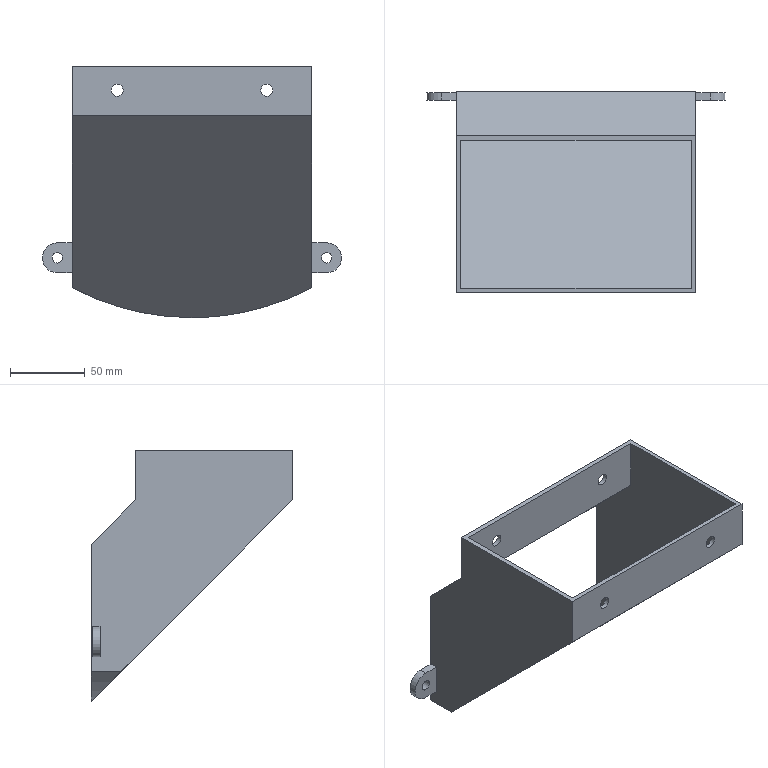Part | NX | features DATUM_CSYS 6, SKETCH 5, EXTRUDE 4, HOLE PACKAGE 4, SIMPLE HOLE 4, BLEND 2, EXTRACT_FACE 2, EXTRACT_STRING 2, DATUM_PLANE 1, Instance Feature 1, Mirror Feature 1, SHELL 1 | 1 solid | 34 faces | box 200 x 135 x 168 mm | volume 211668 mm3 | plane 22 | cylinder 12 | commonest cylinder face diameters 8 x4 7 x2 20 x2 334 x2 340 x2
STEP:
#1=CARTESIAN_POINT('',(160.,135.,-115.));
#2=VERTEX_POINT('',#1);
#3=CARTESIAN_POINT('',(80.,135.,-135.));
#4=VERTEX_POINT('',#3);
#5=CARTESIAN_POINT('',(80.,135.,35.));
#6=DIRECTION('',(0.,-1.,0.));
#7=DIRECTION('',(0.,0.,-1.));
#8=AXIS2_PLACEMENT_3D('',#5,#6,#7);
#9=CIRCLE('',#8,170.);
#10=EDGE_CURVE('',#2,#4,#9,.F.);
#11=ORIENTED_EDGE('',*,*,#10,.T.);
#12=CARTESIAN_POINT('',(0.,135.,-115.));
#13=VERTEX_POINT('',#12);
#14=CARTESIAN_POINT('',(80.,135.,35.));
#15=DIRECTION('',(0.,-1.,0.));
#16=DIRECTION('',(0.,0.,-1.));
#17=AXIS2_PLACEMENT_3D('',#14,#15,#16);
#18=CIRCLE('',#17,170.);
#19=EDGE_CURVE('',#4,#13,#18,.F.);
#20=ORIENTED_EDGE('',*,*,#19,.T.);
#21=CARTESIAN_POINT('',(0.,135.,-30.));
#22=VERTEX_POINT('',#21);
#23=CARTESIAN_POINT('',(0.,135.,-135.));
#24=DIRECTION('',(0.,0.,1.));
#25=VECTOR('',#24,1000.);
#26=LINE('',#23,#25);
#27=EDGE_CURVE('',#13,#22,#26,.T.);
#28=ORIENTED_EDGE('',*,*,#27,.T.);
#29=CARTESIAN_POINT('',(160.,135.,-30.));
#30=VERTEX_POINT('',#29);
#31=CARTESIAN_POINT('',(160.,135.,-30.));
#32=DIRECTION('',(-1.,0.,0.));
#33=VECTOR('',#32,1000.);
#34=LINE('',#31,#33);
#35=EDGE_CURVE('',#30,#22,#34,.T.);
#36=ORIENTED_EDGE('',*,*,#35,.F.);
#37=CARTESIAN_POINT('',(160.,135.,-135.));
#38=DIRECTION('',(0.,0.,1.));
#39=VECTOR('',#38,1000.);
#40=LINE('',#37,#39);
#41=EDGE_CURVE('',#2,#30,#40,.T.);
#42=ORIENTED_EDGE('',*,*,#41,.F.);
#43=EDGE_LOOP('',(#11,#20,#28,#36,#42));
#44=FACE_BOUND('',#43,.T.);
#45=CARTESIAN_POINT('',(157.,135.,-113.189));
#46=VERTEX_POINT('',#45);
#47=CARTESIAN_POINT('',(100.335,135.,-130.757));
#48=VERTEX_POINT('',#47);
#49=CARTESIAN_POINT('',(80.,135.,35.));
#50=DIRECTION('',(0.,-1.,0.));
#51=DIRECTION('',(0.,0.,-1.));
#52=AXIS2_PLACEMENT_3D('',#49,#50,#51);
#53=CIRCLE('',#52,167.);
#54=EDGE_CURVE('',#46,#48,#53,.F.);
#55=ORIENTED_EDGE('',*,*,#54,.F.);
#56=CARTESIAN_POINT('',(157.,135.,-34.243));
#57=VERTEX_POINT('',#56);
#58=CARTESIAN_POINT('',(157.,135.,-135.));
#59=DIRECTION('',(0.,0.,1.));
#60=VECTOR('',#59,1000.);
#61=LINE('',#58,#60);
#62=EDGE_CURVE('',#46,#57,#61,.T.);
#63=ORIENTED_EDGE('',*,*,#62,.T.);
#64=CARTESIAN_POINT('',(3.,135.,-34.243));
#65=VERTEX_POINT('',#64);
#66=CARTESIAN_POINT('',(160.,135.,-34.243));
#67=DIRECTION('',(-1.,0.,0.));
#68=VECTOR('',#67,1000.);
#69=LINE('',#66,#68);
#70=EDGE_CURVE('',#57,#65,#69,.T.);
#71=ORIENTED_EDGE('',*,*,#70,.T.);
#72=CARTESIAN_POINT('',(3.,135.,-113.189));
#73=VERTEX_POINT('',#72);
#74=CARTESIAN_POINT('',(3.,135.,-135.));
#75=DIRECTION('',(0.,0.,1.));
#76=VECTOR('',#75,1000.);
#77=LINE('',#74,#76);
#78=EDGE_CURVE('',#73,#65,#77,.T.);
#79=ORIENTED_EDGE('',*,*,#78,.F.);
#80=CARTESIAN_POINT('',(59.665,135.,-130.757));
#81=VERTEX_POINT('',#80);
#82=CARTESIAN_POINT('',(80.,135.,35.));
#83=DIRECTION('',(0.,-1.,0.));
#84=DIRECTION('',(0.,0.,-1.));
#85=AXIS2_PLACEMENT_3D('',#82,#83,#84);
#86=CIRCLE('',#85,167.);
#87=EDGE_CURVE('',#81,#73,#86,.F.);
#88=ORIENTED_EDGE('',*,*,#87,.F.);
#89=CARTESIAN_POINT('',(160.,135.,-130.757));
#90=DIRECTION('',(-1.,0.,0.));
#91=VECTOR('',#90,1000.);
#92=LINE('',#89,#91);
#93=EDGE_CURVE('',#48,#81,#92,.T.);
#94=ORIENTED_EDGE('',*,*,#93,.F.);
#95=EDGE_LOOP('',(#55,#63,#71,#79,#88,#94));
#96=FACE_BOUND('',#95,.T.);
#97=CARTESIAN_POINT('',(160.,135.,-135.));
#98=DIRECTION('',(0.,-1.,0.));
#99=DIRECTION('',(0.,0.,-1.));
#100=AXIS2_PLACEMENT_3D('',#97,#98,#99);
#101=PLANE('',#100);
#102=ADVANCED_FACE('',(#44,#96),#101,.F.);
#103=CARTESIAN_POINT('',(0.,105.,33.));
#104=VERTEX_POINT('',#103);
#105=CARTESIAN_POINT('',(0.,0.,33.));
#106=VERTEX_POINT('',#105);
#107=CARTESIAN_POINT('',(0.,105.,33.));
#108=DIRECTION('',(0.,-1.,0.));
#109=VECTOR('',#108,1000.);
#110=LINE('',#107,#109);
#111=EDGE_CURVE('',#104,#106,#110,.T.);
#112=ORIENTED_EDGE('',*,*,#111,.T.);
#113=CARTESIAN_POINT('',(160.,0.,33.));
#114=VERTEX_POINT('',#113);
#115=CARTESIAN_POINT('',(160.,0.,33.));
#116=DIRECTION('',(-1.,0.,0.));
#117=VECTOR('',#116,1000.);
#118=LINE('',#115,#117);
#119=EDGE_CURVE('',#114,#106,#118,.T.);
#120=ORIENTED_EDGE('',*,*,#119,.F.);
#121=CARTESIAN_POINT('',(160.,105.,33.));
#122=VERTEX_POINT('',#121);
#123=CARTESIAN_POINT('',(160.,105.,33.));
#124=DIRECTION('',(0.,-1.,0.));
#125=VECTOR('',#124,1000.);
#126=LINE('',#123,#125);
#127=EDGE_CURVE('',#122,#114,#126,.T.);
#128=ORIENTED_EDGE('',*,*,#127,.F.);
#129=CARTESIAN_POINT('',(160.,105.,33.));
#130=DIRECTION('',(-1.,0.,0.));
#131=VECTOR('',#130,1000.);
#132=LINE('',#129,#131);
#133=EDGE_CURVE('',#122,#104,#132,.T.);
#134=ORIENTED_EDGE('',*,*,#133,.T.);
#135=EDGE_LOOP('',(#112,#120,#128,#134));
#136=FACE_BOUND('',#135,.T.);
#137=CARTESIAN_POINT('',(3.,102.,33.));
#138=VERTEX_POINT('',#137);
#139=CARTESIAN_POINT('',(3.,3.,33.));
#140=VERTEX_POINT('',#139);
#141=CARTESIAN_POINT('',(3.,105.,33.));
#142=DIRECTION('',(0.,-1.,0.));
#143=VECTOR('',#142,1000.);
#144=LINE('',#141,#143);
#145=EDGE_CURVE('',#138,#140,#144,.T.);
#146=ORIENTED_EDGE('',*,*,#145,.F.);
#147=CARTESIAN_POINT('',(157.,102.,33.));
#148=VERTEX_POINT('',#147);
#149=CARTESIAN_POINT('',(160.,102.,33.));
#150=DIRECTION('',(-1.,0.,0.));
#151=VECTOR('',#150,1000.);
#152=LINE('',#149,#151);
#153=EDGE_CURVE('',#148,#138,#152,.T.);
#154=ORIENTED_EDGE('',*,*,#153,.F.);
#155=CARTESIAN_POINT('',(157.,3.,33.));
#156=VERTEX_POINT('',#155);
#157=CARTESIAN_POINT('',(157.,105.,33.));
#158=DIRECTION('',(0.,-1.,0.));
#159=VECTOR('',#158,1000.);
#160=LINE('',#157,#159);
#161=EDGE_CURVE('',#148,#156,#160,.T.);
#162=ORIENTED_EDGE('',*,*,#161,.T.);
#163=CARTESIAN_POINT('',(160.,3.,33.));
#164=DIRECTION('',(-1.,0.,0.));
#165=VECTOR('',#164,1000.);
#166=LINE('',#163,#165);
#167=EDGE_CURVE('',#156,#140,#166,.T.);
#168=ORIENTED_EDGE('',*,*,#167,.T.);
#169=EDGE_LOOP('',(#146,#154,#162,#168));
#170=FACE_BOUND('',#169,.T.);
#171=CARTESIAN_POINT('',(160.,105.,33.));
#172=DIRECTION('',(0.,0.,-1.));
#173=DIRECTION('',(-1.,0.,0.));
#174=AXIS2_PLACEMENT_3D('',#171,#172,#173);
#175=PLANE('',#174);
#176=ADVANCED_FACE('',(#136,#170),#175,.F.);
#177=CARTESIAN_POINT('',(130.,3.,21.));
#178=VERTEX_POINT('',#177);
#179=CARTESIAN_POINT('',(130.,3.,17.));
#180=DIRECTION('',(0.,1.,0.));
#181=DIRECTION('',(0.,0.,1.));
#182=AXIS2_PLACEMENT_3D('',#179,#180,#181);
#183=CIRCLE('',#182,4.);
#184=EDGE_CURVE('',#178,#178,#183,.T.);
#185=ORIENTED_EDGE('',*,*,#184,.T.);
#186=EDGE_LOOP('',(#185));
#187=FACE_BOUND('',#186,.T.);
#188=CARTESIAN_POINT('',(130.,0.,21.));
#189=VERTEX_POINT('',#188);
#190=CARTESIAN_POINT('',(130.,0.,17.));
#191=DIRECTION('',(0.,1.,0.));
#192=DIRECTION('',(0.,0.,1.));
#193=AXIS2_PLACEMENT_3D('',#190,#191,#192);
#194=CIRCLE('',#193,4.);
#195=EDGE_CURVE('',#189,#189,#194,.T.);
#196=ORIENTED_EDGE('',*,*,#195,.F.);
#197=EDGE_LOOP('',(#196));
#198=FACE_BOUND('',#197,.T.);
#199=CARTESIAN_POINT('',(130.,0.,17.));
#200=DIRECTION('',(0.,1.,0.));
#201=DIRECTION('',(0.,0.,1.));
#202=AXIS2_PLACEMENT_3D('',#199,#200,#201);
#203=CYLINDRICAL_SURFACE('',#202,4.);
#204=ADVANCED_FACE('',(#187,#198),#203,.F.);
#205=CARTESIAN_POINT('',(30.,3.,21.));
#206=VERTEX_POINT('',#205);
#207=CARTESIAN_POINT('',(30.,3.,17.));
#208=DIRECTION('',(0.,1.,0.));
#209=DIRECTION('',(0.,0.,1.));
#210=AXIS2_PLACEMENT_3D('',#207,#208,#209);
#211=CIRCLE('',#210,4.);
#212=EDGE_CURVE('',#206,#206,#211,.T.);
#213=ORIENTED_EDGE('',*,*,#212,.T.);
#214=EDGE_LOOP('',(#213));
#215=FACE_BOUND('',#214,.T.);
#216=CARTESIAN_POINT('',(30.,0.,21.));
#217=VERTEX_POINT('',#216);
#218=CARTESIAN_POINT('',(30.,0.,17.));
#219=DIRECTION('',(0.,1.,0.));
#220=DIRECTION('',(0.,0.,1.));
#221=AXIS2_PLACEMENT_3D('',#218,#219,#220);
#222=CIRCLE('',#221,4.);
#223=EDGE_CURVE('',#217,#217,#222,.T.);
#224=ORIENTED_EDGE('',*,*,#223,.F.);
#225=EDGE_LOOP('',(#224));
#226=FACE_BOUND('',#225,.T.);
#227=CARTESIAN_POINT('',(30.,0.,17.));
#228=DIRECTION('',(0.,1.,0.));
#229=DIRECTION('',(0.,0.,1.));
#230=AXIS2_PLACEMENT_3D('',#227,#228,#229);
#231=CYLINDRICAL_SURFACE('',#230,4.);
#232=ADVANCED_FACE('',(#215,#226),#231,.F.);
#233=CARTESIAN_POINT('',(0.,0.,0.));
#234=VERTEX_POINT('',#233);
#235=CARTESIAN_POINT('',(0.,115.,-115.));
#236=VERTEX_POINT('',#235);
#237=CARTESIAN_POINT('',(0.,0.,0.));
#238=DIRECTION('',(0.,0.7071,-0.7071));
#239=VECTOR('',#238,1000.);
#240=LINE('',#237,#239);
#241=EDGE_CURVE('',#234,#236,#240,.T.);
#242=ORIENTED_EDGE('',*,*,#241,.T.);
#243=CARTESIAN_POINT('',(80.,-35.,35.));
#244=DIRECTION('',(0.,0.7071,0.7071));
#245=DIRECTION('',(0.,-0.7071,0.7071));
#246=AXIS2_PLACEMENT_3D('',#243,#244,#245);
#247=ELLIPSE('',#246,240.416,170.);
#248=EDGE_CURVE('',#236,#4,#247,.F.);
#249=ORIENTED_EDGE('',*,*,#248,.T.);
#250=CARTESIAN_POINT('',(160.,115.,-115.));
#251=VERTEX_POINT('',#250);
#252=CARTESIAN_POINT('',(80.,-35.,35.));
#253=DIRECTION('',(0.,0.7071,0.7071));
#254=DIRECTION('',(0.,-0.7071,0.7071));
#255=AXIS2_PLACEMENT_3D('',#252,#253,#254);
#256=ELLIPSE('',#255,240.416,170.);
#257=EDGE_CURVE('',#4,#251,#256,.F.);
#258=ORIENTED_EDGE('',*,*,#257,.T.);
#259=CARTESIAN_POINT('',(160.,0.,0.));
#260=VERTEX_POINT('',#259);
#261=CARTESIAN_POINT('',(160.,0.,0.));
#262=DIRECTION('',(0.,0.7071,-0.7071));
#263=VECTOR('',#262,1000.);
#264=LINE('',#261,#263);
#265=EDGE_CURVE('',#260,#251,#264,.T.);
#266=ORIENTED_EDGE('',*,*,#265,.F.);
#267=CARTESIAN_POINT('',(160.,0.,0.));
#268=DIRECTION('',(-1.,0.,0.));
#269=VECTOR('',#268,1000.);
#270=LINE('',#267,#269);
#271=EDGE_CURVE('',#260,#234,#270,.T.);
#272=ORIENTED_EDGE('',*,*,#271,.T.);
#273=EDGE_LOOP('',(#242,#249,#258,#266,#272));
#274=FACE_BOUND('',#273,.T.);
#275=CARTESIAN_POINT('',(160.,0.,0.));
#276=DIRECTION('',(0.,0.7071,0.7071));
#277=DIRECTION('',(0.,-0.7071,0.7071));
#278=AXIS2_PLACEMENT_3D('',#275,#276,#277);
#279=PLANE('',#278);
#280=ADVANCED_FACE('',(#274),#279,.F.);
#281=ORIENTED_EDGE('',*,*,#27,.F.);
#282=CARTESIAN_POINT('',(0.,275.,-115.));
#283=DIRECTION('',(0.,-1.,0.));
#284=VECTOR('',#283,1000.);
#285=LINE('',#282,#284);
#286=EDGE_CURVE('',#13,#236,#285,.T.);
#287=ORIENTED_EDGE('',*,*,#286,.T.);
#288=ORIENTED_EDGE('',*,*,#241,.F.);
#289=CARTESIAN_POINT('',(0.,0.,33.));
#290=DIRECTION('',(0.,0.,-1.));
#291=VECTOR('',#290,1000.);
#292=LINE('',#289,#291);
#293=EDGE_CURVE('',#106,#234,#292,.T.);
#294=ORIENTED_EDGE('',*,*,#293,.F.);
#295=ORIENTED_EDGE('',*,*,#111,.F.);
#296=CARTESIAN_POINT('',(0.,105.,0.));
#297=VERTEX_POINT('',#296);
#298=CARTESIAN_POINT('',(0.,105.,0.));
#299=DIRECTION('',(0.,0.,1.));
#300=VECTOR('',#299,1000.);
#301=LINE('',#298,#300);
#302=EDGE_CURVE('',#297,#104,#301,.T.);
#303=ORIENTED_EDGE('',*,*,#302,.F.);
#304=CARTESIAN_POINT('',(0.,135.,-30.));
#305=DIRECTION('',(0.,-0.7071,0.7071));
#306=VECTOR('',#305,1000.);
#307=LINE('',#304,#306);
#308=EDGE_CURVE('',#22,#297,#307,.T.);
#309=ORIENTED_EDGE('',*,*,#308,.F.);
#310=EDGE_LOOP('',(#281,#287,#288,#294,#295,#303,#309));
#311=FACE_BOUND('',#310,.T.);
#312=CARTESIAN_POINT('',(0.,134.,-85.));
#313=VERTEX_POINT('',#312);
#314=CARTESIAN_POINT('',(0.,134.,-105.));
#315=VERTEX_POINT('',#314);
#316=CARTESIAN_POINT('',(0.,134.,-85.));
#317=DIRECTION('',(0.,0.,-1.));
#318=VECTOR('',#317,1000.);
#319=LINE('',#316,#318);
#320=EDGE_CURVE('',#313,#315,#319,.T.);
#321=ORIENTED_EDGE('',*,*,#320,.F.);
#322=CARTESIAN_POINT('',(0.,129.,-85.));
#323=VERTEX_POINT('',#322);
#324=CARTESIAN_POINT('',(0.,129.,-85.));
#325=DIRECTION('',(0.,1.,0.));
#326=VECTOR('',#325,1000.);
#327=LINE('',#324,#326);
#328=EDGE_CURVE('',#323,#313,#327,.T.);
#329=ORIENTED_EDGE('',*,*,#328,.F.);
#330=CARTESIAN_POINT('',(0.,129.,-105.));
#331=VERTEX_POINT('',#330);
#332=CARTESIAN_POINT('',(0.,129.,-85.));
#333=DIRECTION('',(0.,0.,-1.));
#334=VECTOR('',#333,1000.);
#335=LINE('',#332,#334);
#336=EDGE_CURVE('',#323,#331,#335,.T.);
#337=ORIENTED_EDGE('',*,*,#336,.T.);
#338=CARTESIAN_POINT('',(0.,129.,-105.));
#339=DIRECTION('',(0.,1.,0.));
#340=VECTOR('',#339,1000.);
#341=LINE('',#338,#340);
#342=EDGE_CURVE('',#331,#315,#341,.T.);
#343=ORIENTED_EDGE('',*,*,#342,.T.);
#344=EDGE_LOOP('',(#321,#329,#337,#343));
#345=FACE_BOUND('',#344,.T.);
#346=CARTESIAN_POINT('',(0.,0.,0.));
#347=DIRECTION('',(1.,0.,0.));
#348=DIRECTION('',(0.,0.,-1.));
#349=AXIS2_PLACEMENT_3D('',#346,#347,#348);
#350=PLANE('',#349);
#351=ADVANCED_FACE('',(#311,#345),#350,.F.);
#352=CARTESIAN_POINT('',(160.,275.,-115.));
#353=DIRECTION('',(0.,-1.,0.));
#354=VECTOR('',#353,1000.);
#355=LINE('',#352,#354);
#356=EDGE_CURVE('',#2,#251,#355,.T.);
#357=ORIENTED_EDGE('',*,*,#356,.F.);
#358=ORIENTED_EDGE('',*,*,#41,.T.);
#359=CARTESIAN_POINT('',(160.,105.,0.));
#360=VERTEX_POINT('',#359);
#361=CARTESIAN_POINT('',(160.,135.,-30.));
#362=DIRECTION('',(0.,-0.7071,0.7071));
#363=VECTOR('',#362,1000.);
#364=LINE('',#361,#363);
#365=EDGE_CURVE('',#30,#360,#364,.T.);
#366=ORIENTED_EDGE('',*,*,#365,.T.);
#367=CARTESIAN_POINT('',(160.,105.,0.));
#368=DIRECTION('',(0.,0.,1.));
#369=VECTOR('',#368,1000.);
#370=LINE('',#367,#369);
#371=EDGE_CURVE('',#360,#122,#370,.T.);
#372=ORIENTED_EDGE('',*,*,#371,.T.);
#373=ORIENTED_EDGE('',*,*,#127,.T.);
#374=CARTESIAN_POINT('',(160.,0.,33.));
#375=DIRECTION('',(0.,0.,-1.));
#376=VECTOR('',#375,1000.);
#377=LINE('',#374,#376);
#378=EDGE_CURVE('',#114,#260,#377,.T.);
#379=ORIENTED_EDGE('',*,*,#378,.T.);
#380=ORIENTED_EDGE('',*,*,#265,.T.);
#381=EDGE_LOOP('',(#357,#358,#366,#372,#373,#379,#380));
#382=FACE_BOUND('',#381,.T.);
#383=CARTESIAN_POINT('',(160.,129.,-85.));
#384=VERTEX_POINT('',#383);
#385=CARTESIAN_POINT('',(160.,134.,-85.));
#386=VERTEX_POINT('',#385);
#387=CARTESIAN_POINT('',(160.,129.,-85.));
#388=DIRECTION('',(0.,1.,0.));
#389=VECTOR('',#388,1000.);
#390=LINE('',#387,#389);
#391=EDGE_CURVE('',#384,#386,#390,.T.);
#392=ORIENTED_EDGE('',*,*,#391,.T.);
#393=CARTESIAN_POINT('',(160.,134.,-105.));
#394=VERTEX_POINT('',#393);
#395=CARTESIAN_POINT('',(160.,134.,-85.));
#396=DIRECTION('',(0.,0.,-1.));
#397=VECTOR('',#396,1000.);
#398=LINE('',#395,#397);
#399=EDGE_CURVE('',#386,#394,#398,.T.);
#400=ORIENTED_EDGE('',*,*,#399,.T.);
#401=CARTESIAN_POINT('',(160.,129.,-105.));
#402=VERTEX_POINT('',#401);
#403=CARTESIAN_POINT('',(160.,129.,-105.));
#404=DIRECTION('',(0.,1.,0.));
#405=VECTOR('',#404,1000.);
#406=LINE('',#403,#405);
#407=EDGE_CURVE('',#402,#394,#406,.T.);
#408=ORIENTED_EDGE('',*,*,#407,.F.);
#409=CARTESIAN_POINT('',(160.,129.,-85.));
#410=DIRECTION('',(0.,0.,-1.));
#411=VECTOR('',#410,1000.);
#412=LINE('',#409,#411);
#413=EDGE_CURVE('',#384,#402,#412,.T.);
#414=ORIENTED_EDGE('',*,*,#413,.F.);
#415=EDGE_LOOP('',(#392,#400,#408,#414));
#416=FACE_BOUND('',#415,.T.);
#417=CARTESIAN_POINT('',(160.,0.,0.));
#418=DIRECTION('',(1.,0.,0.));
#419=DIRECTION('',(0.,0.,-1.));
#420=AXIS2_PLACEMENT_3D('',#417,#418,#419);
#421=PLANE('',#420);
#422=ADVANCED_FACE('',(#382,#416),#421,.T.);
#423=ORIENTED_EDGE('',*,*,#223,.T.);
#424=EDGE_LOOP('',(#423));
#425=FACE_BOUND('',#424,.T.);
#426=ORIENTED_EDGE('',*,*,#195,.T.);
#427=EDGE_LOOP('',(#426));
#428=FACE_BOUND('',#427,.T.);
#429=ORIENTED_EDGE('',*,*,#293,.T.);
#430=ORIENTED_EDGE('',*,*,#271,.F.);
#431=ORIENTED_EDGE('',*,*,#378,.F.);
#432=ORIENTED_EDGE('',*,*,#119,.T.);
#433=EDGE_LOOP('',(#429,#430,#431,#432));
#434=FACE_BOUND('',#433,.T.);
#435=CARTESIAN_POINT('',(160.,0.,33.));
#436=DIRECTION('',(0.,1.,0.));
#437=DIRECTION('',(0.,0.,1.));
#438=AXIS2_PLACEMENT_3D('',#435,#436,#437);
#439=PLANE('',#438);
#440=ADVANCED_FACE('',(#425,#428,#434),#439,.F.);
#441=ORIENTED_EDGE('',*,*,#308,.T.);
#442=CARTESIAN_POINT('',(160.,105.,0.));
#443=DIRECTION('',(-1.,0.,0.));
#444=VECTOR('',#443,1000.);
#445=LINE('',#442,#444);
#446=EDGE_CURVE('',#360,#297,#445,.T.);
#447=ORIENTED_EDGE('',*,*,#446,.F.);
#448=ORIENTED_EDGE('',*,*,#365,.F.);
#449=ORIENTED_EDGE('',*,*,#35,.T.);
#450=EDGE_LOOP('',(#441,#447,#448,#449));
#451=FACE_BOUND('',#450,.T.);
#452=CARTESIAN_POINT('',(160.,135.,-30.));
#453=DIRECTION('',(0.,-0.7071,-0.7071));
#454=DIRECTION('',(0.,0.7071,-0.7071));
#455=AXIS2_PLACEMENT_3D('',#452,#453,#454);
#456=PLANE('',#455);
#457=ADVANCED_FACE('',(#451),#456,.F.);
#458=CARTESIAN_POINT('',(30.,105.,13.));
#459=VERTEX_POINT('',#458);
#460=CARTESIAN_POINT('',(30.,105.,17.));
#461=DIRECTION('',(0.,-1.,0.));
#462=DIRECTION('',(0.,0.,-1.));
#463=AXIS2_PLACEMENT_3D('',#460,#461,#462);
#464=CIRCLE('',#463,4.);
#465=EDGE_CURVE('',#459,#459,#464,.T.);
#466=ORIENTED_EDGE('',*,*,#465,.T.);
#467=EDGE_LOOP('',(#466));
#468=FACE_BOUND('',#467,.T.);
#469=CARTESIAN_POINT('',(130.,105.,13.));
#470=VERTEX_POINT('',#469);
#471=CARTESIAN_POINT('',(130.,105.,17.));
#472=DIRECTION('',(0.,-1.,0.));
#473=DIRECTION('',(0.,0.,-1.));
#474=AXIS2_PLACEMENT_3D('',#471,#472,#473);
#475=CIRCLE('',#474,4.);
#476=EDGE_CURVE('',#470,#470,#475,.T.);
#477=ORIENTED_EDGE('',*,*,#476,.T.);
#478=EDGE_LOOP('',(#477));
#479=FACE_BOUND('',#478,.T.);
#480=ORIENTED_EDGE('',*,*,#302,.T.);
#481=ORIENTED_EDGE('',*,*,#133,.F.);
#482=ORIENTED_EDGE('',*,*,#371,.F.);
#483=ORIENTED_EDGE('',*,*,#446,.T.);
#484=EDGE_LOOP('',(#480,#481,#482,#483));
#485=FACE_BOUND('',#484,.T.);
#486=CARTESIAN_POINT('',(160.,105.,0.));
#487=DIRECTION('',(0.,-1.,0.));
#488=DIRECTION('',(0.,0.,-1.));
#489=AXIS2_PLACEMENT_3D('',#486,#487,#488);
#490=PLANE('',#489);
#491=ADVANCED_FACE('',(#468,#479,#485),#490,.F.);
#492=CARTESIAN_POINT('',(170.,129.,-85.));
#493=VERTEX_POINT('',#492);
#494=CARTESIAN_POINT('',(180.,129.,-85.));
#495=DIRECTION('',(-1.,0.,0.));
#496=VECTOR('',#495,1000.);
#497=LINE('',#494,#496);
#498=EDGE_CURVE('',#493,#384,#497,.T.);
#499=ORIENTED_EDGE('',*,*,#498,.F.);
#500=CARTESIAN_POINT('',(170.,134.,-85.));
#501=VERTEX_POINT('',#500);
#502=CARTESIAN_POINT('',(170.,129.,-85.));
#503=DIRECTION('',(0.,1.,0.));
#504=VECTOR('',#503,1000.);
#505=LINE('',#502,#504);
#506=EDGE_CURVE('',#493,#501,#505,.T.);
#507=ORIENTED_EDGE('',*,*,#506,.T.);
#508=CARTESIAN_POINT('',(180.,134.,-85.));
#509=DIRECTION('',(-1.,0.,0.));
#510=VECTOR('',#509,1000.);
#511=LINE('',#508,#510);
#512=EDGE_CURVE('',#501,#386,#511,.T.);
#513=ORIENTED_EDGE('',*,*,#512,.T.);
#514=ORIENTED_EDGE('',*,*,#391,.F.);
#515=EDGE_LOOP('',(#499,#507,#513,#514));
#516=FACE_BOUND('',#515,.T.);
#517=CARTESIAN_POINT('',(180.,129.,-85.));
#518=DIRECTION('',(0.,0.,-1.));
#519=DIRECTION('',(-1.,0.,0.));
#520=AXIS2_PLACEMENT_3D('',#517,#518,#519);
#521=PLANE('',#520);
#522=ADVANCED_FACE('',(#516),#521,.F.);
#523=CARTESIAN_POINT('',(170.,134.,-105.));
#524=VERTEX_POINT('',#523);
#525=CARTESIAN_POINT('',(160.,134.,-105.));
#526=DIRECTION('',(1.,0.,0.));
#527=VECTOR('',#526,1000.);
#528=LINE('',#525,#527);
#529=EDGE_CURVE('',#394,#524,#528,.T.);
#530=ORIENTED_EDGE('',*,*,#529,.T.);
#531=CARTESIAN_POINT('',(170.,129.,-105.));
#532=VERTEX_POINT('',#531);
#533=CARTESIAN_POINT('',(170.,129.,-105.));
#534=DIRECTION('',(0.,1.,0.));
#535=VECTOR('',#534,1000.);
#536=LINE('',#533,#535);
#537=EDGE_CURVE('',#524,#532,#536,.F.);
#538=ORIENTED_EDGE('',*,*,#537,.T.);
#539=CARTESIAN_POINT('',(160.,129.,-105.));
#540=DIRECTION('',(1.,0.,0.));
#541=VECTOR('',#540,1000.);
#542=LINE('',#539,#541);
#543=EDGE_CURVE('',#402,#532,#542,.T.);
#544=ORIENTED_EDGE('',*,*,#543,.F.);
#545=ORIENTED_EDGE('',*,*,#407,.T.);
#546=EDGE_LOOP('',(#530,#538,#544,#545));
#547=FACE_BOUND('',#546,.T.);
#548=CARTESIAN_POINT('',(160.,129.,-105.));
#549=DIRECTION('',(0.,0.,1.));
#550=DIRECTION('',(1.,0.,0.));
#551=AXIS2_PLACEMENT_3D('',#548,#549,#550);
#552=PLANE('',#551);
#553=ADVANCED_FACE('',(#547),#552,.F.);
#554=CARTESIAN_POINT('',(170.,129.,-98.5));
#555=VERTEX_POINT('',#554);
#556=CARTESIAN_POINT('',(170.,129.,-95.));
#557=DIRECTION('',(0.,-1.,0.));
#558=DIRECTION('',(0.,0.,-1.));
#559=AXIS2_PLACEMENT_3D('',#556,#557,#558);
#560=CIRCLE('',#559,3.5);
#561=EDGE_CURVE('',#555,#555,#560,.T.);
#562=ORIENTED_EDGE('',*,*,#561,.F.);
#563=EDGE_LOOP('',(#562));
#564=FACE_BOUND('',#563,.T.);
#565=CARTESIAN_POINT('',(170.,129.,-95.));
#566=DIRECTION('',(0.,-1.,0.));
#567=DIRECTION('',(0.,0.,-1.));
#568=AXIS2_PLACEMENT_3D('',#565,#566,#567);
#569=CIRCLE('',#568,10.);
#570=EDGE_CURVE('',#532,#493,#569,.T.);
#571=ORIENTED_EDGE('',*,*,#570,.T.);
#572=ORIENTED_EDGE('',*,*,#498,.T.);
#573=ORIENTED_EDGE('',*,*,#413,.T.);
#574=ORIENTED_EDGE('',*,*,#543,.T.);
#575=EDGE_LOOP('',(#571,#572,#573,#574));
#576=FACE_BOUND('',#575,.T.);
#577=CARTESIAN_POINT('',(0.,129.,0.));
#578=DIRECTION('',(0.,-1.,0.));
#579=DIRECTION('',(0.,0.,-1.));
#580=AXIS2_PLACEMENT_3D('',#577,#578,#579);
#581=PLANE('',#580);
#582=ADVANCED_FACE('',(#564,#576),#581,.T.);
#583=CARTESIAN_POINT('',(170.,134.,-98.5));
#584=VERTEX_POINT('',#583);
#585=CARTESIAN_POINT('',(170.,134.,-95.));
#586=DIRECTION('',(0.,-1.,0.));
#587=DIRECTION('',(0.,0.,-1.));
#588=AXIS2_PLACEMENT_3D('',#585,#586,#587);
#589=CIRCLE('',#588,3.5);
#590=EDGE_CURVE('',#584,#584,#589,.T.);
#591=ORIENTED_EDGE('',*,*,#590,.T.);
#592=EDGE_LOOP('',(#591));
#593=FACE_BOUND('',#592,.T.);
#594=ORIENTED_EDGE('',*,*,#512,.F.);
#595=CARTESIAN_POINT('',(170.,134.,-95.));
#596=DIRECTION('',(0.,-1.,0.));
#597=DIRECTION('',(0.,0.,-1.));
#598=AXIS2_PLACEMENT_3D('',#595,#596,#597);
#599=CIRCLE('',#598,10.);
#600=EDGE_CURVE('',#501,#524,#599,.F.);
#601=ORIENTED_EDGE('',*,*,#600,.T.);
#602=ORIENTED_EDGE('',*,*,#529,.F.);
#603=ORIENTED_EDGE('',*,*,#399,.F.);
#604=EDGE_LOOP('',(#594,#601,#602,#603));
#605=FACE_BOUND('',#604,.T.);
#606=CARTESIAN_POINT('',(0.,134.,0.));
#607=DIRECTION('',(0.,-1.,0.));
#608=DIRECTION('',(0.,0.,-1.));
#609=AXIS2_PLACEMENT_3D('',#606,#607,#608);
#610=PLANE('',#609);
#611=ADVANCED_FACE('',(#593,#605),#610,.F.);
#612=ORIENTED_EDGE('',*,*,#600,.F.);
#613=ORIENTED_EDGE('',*,*,#506,.F.);
#614=ORIENTED_EDGE('',*,*,#570,.F.);
#615=ORIENTED_EDGE('',*,*,#537,.F.);
#616=EDGE_LOOP('',(#612,#613,#614,#615));
#617=FACE_BOUND('',#616,.T.);
#618=CARTESIAN_POINT('',(170.,129.,-95.));
#619=DIRECTION('',(0.,1.,0.));
#620=DIRECTION('',(0.,0.,1.));
#621=AXIS2_PLACEMENT_3D('',#618,#619,#620);
#622=CYLINDRICAL_SURFACE('',#621,10.);
#623=ADVANCED_FACE('',(#617),#622,.T.);
#624=ORIENTED_EDGE('',*,*,#561,.T.);
#625=EDGE_LOOP('',(#624));
#626=FACE_BOUND('',#625,.T.);
#627=ORIENTED_EDGE('',*,*,#590,.F.);
#628=EDGE_LOOP('',(#627));
#629=FACE_BOUND('',#628,.T.);
#630=CARTESIAN_POINT('',(170.,134.,-95.));
#631=DIRECTION('',(0.,-1.,0.));
#632=DIRECTION('',(0.,0.,-1.));
#633=AXIS2_PLACEMENT_3D('',#630,#631,#632);
#634=CYLINDRICAL_SURFACE('',#633,3.5);
#635=ADVANCED_FACE('',(#626,#629),#634,.F.);
#636=CARTESIAN_POINT('',(130.,102.,13.));
#637=VERTEX_POINT('',#636);
#638=CARTESIAN_POINT('',(130.,102.,17.));
#639=DIRECTION('',(0.,-1.,0.));
#640=DIRECTION('',(0.,0.,-1.));
#641=AXIS2_PLACEMENT_3D('',#638,#639,#640);
#642=CIRCLE('',#641,4.);
#643=EDGE_CURVE('',#637,#637,#642,.T.);
#644=ORIENTED_EDGE('',*,*,#643,.T.);
#645=EDGE_LOOP('',(#644));
#646=FACE_BOUND('',#645,.T.);
#647=ORIENTED_EDGE('',*,*,#476,.F.);
#648=EDGE_LOOP('',(#647));
#649=FACE_BOUND('',#648,.T.);
#650=CARTESIAN_POINT('',(130.,0.,17.));
#651=DIRECTION('',(0.,1.,0.));
#652=DIRECTION('',(0.,0.,1.));
#653=AXIS2_PLACEMENT_3D('',#650,#651,#652);
#654=CYLINDRICAL_SURFACE('',#653,4.);
#655=ADVANCED_FACE('',(#646,#649),#654,.F.);
#656=CARTESIAN_POINT('',(-10.,134.,-85.));
#657=VERTEX_POINT('',#656);
#658=CARTESIAN_POINT('',(-20.,134.,-85.));
#659=DIRECTION('',(1.,0.,0.));
#660=VECTOR('',#659,1000.);
#661=LINE('',#658,#660);
#662=EDGE_CURVE('',#657,#313,#661,.T.);
#663=ORIENTED_EDGE('',*,*,#662,.F.);
#664=CARTESIAN_POINT('',(-10.,129.,-85.));
#665=VERTEX_POINT('',#664);
#666=CARTESIAN_POINT('',(-10.,129.,-85.));
#667=DIRECTION('',(0.,1.,0.));
#668=VECTOR('',#667,1000.);
#669=LINE('',#666,#668);
#670=EDGE_CURVE('',#665,#657,#669,.T.);
#671=ORIENTED_EDGE('',*,*,#670,.F.);
#672=CARTESIAN_POINT('',(-20.,129.,-85.));
#673=DIRECTION('',(1.,0.,0.));
#674=VECTOR('',#673,1000.);
#675=LINE('',#672,#674);
#676=EDGE_CURVE('',#665,#323,#675,.T.);
#677=ORIENTED_EDGE('',*,*,#676,.T.);
#678=ORIENTED_EDGE('',*,*,#328,.T.);
#679=EDGE_LOOP('',(#663,#671,#677,#678));
#680=FACE_BOUND('',#679,.T.);
#681=CARTESIAN_POINT('',(-20.,129.,-85.));
#682=DIRECTION('',(0.,0.,1.));
#683=DIRECTION('',(1.,0.,0.));
#684=AXIS2_PLACEMENT_3D('',#681,#682,#683);
#685=PLANE('',#684);
#686=ADVANCED_FACE('',(#680),#685,.T.);
#687=CARTESIAN_POINT('',(-10.,129.,-105.));
#688=VERTEX_POINT('',#687);
#689=CARTESIAN_POINT('',(0.,129.,-105.));
#690=DIRECTION('',(-1.,0.,0.));
#691=VECTOR('',#690,1000.);
#692=LINE('',#689,#691);
#693=EDGE_CURVE('',#331,#688,#692,.T.);
#694=ORIENTED_EDGE('',*,*,#693,.T.);
#695=CARTESIAN_POINT('',(-10.,134.,-105.));
#696=VERTEX_POINT('',#695);
#697=CARTESIAN_POINT('',(-10.,129.,-105.));
#698=DIRECTION('',(0.,1.,0.));
#699=VECTOR('',#698,1000.);
#700=LINE('',#697,#699);
#701=EDGE_CURVE('',#696,#688,#700,.F.);
#702=ORIENTED_EDGE('',*,*,#701,.F.);
#703=CARTESIAN_POINT('',(0.,134.,-105.));
#704=DIRECTION('',(-1.,0.,0.));
#705=VECTOR('',#704,1000.);
#706=LINE('',#703,#705);
#707=EDGE_CURVE('',#315,#696,#706,.T.);
#708=ORIENTED_EDGE('',*,*,#707,.F.);
#709=ORIENTED_EDGE('',*,*,#342,.F.);
#710=EDGE_LOOP('',(#694,#702,#708,#709));
#711=FACE_BOUND('',#710,.T.);
#712=CARTESIAN_POINT('',(0.,129.,-105.));
#713=DIRECTION('',(0.,0.,-1.));
#714=DIRECTION('',(-1.,0.,0.));
#715=AXIS2_PLACEMENT_3D('',#712,#713,#714);
#716=PLANE('',#715);
#717=ADVANCED_FACE('',(#711),#716,.T.);
#718=CARTESIAN_POINT('',(-10.,129.,-91.5));
#719=VERTEX_POINT('',#718);
#720=CARTESIAN_POINT('',(-10.,129.,-95.));
#721=DIRECTION('',(0.,1.,0.));
#722=DIRECTION('',(0.,0.,1.));
#723=AXIS2_PLACEMENT_3D('',#720,#721,#722);
#724=CIRCLE('',#723,3.5);
#725=EDGE_CURVE('',#719,#719,#724,.T.);
#726=ORIENTED_EDGE('',*,*,#725,.T.);
#727=EDGE_LOOP('',(#726));
#728=FACE_BOUND('',#727,.T.);
#729=ORIENTED_EDGE('',*,*,#676,.F.);
#730=CARTESIAN_POINT('',(-10.,129.,-95.));
#731=DIRECTION('',(0.,1.,0.));
#732=DIRECTION('',(0.,0.,1.));
#733=AXIS2_PLACEMENT_3D('',#730,#731,#732);
#734=CIRCLE('',#733,10.);
#735=EDGE_CURVE('',#688,#665,#734,.T.);
#736=ORIENTED_EDGE('',*,*,#735,.F.);
#737=ORIENTED_EDGE('',*,*,#693,.F.);
#738=ORIENTED_EDGE('',*,*,#336,.F.);
#739=EDGE_LOOP('',(#729,#736,#737,#738));
#740=FACE_BOUND('',#739,.T.);
#741=CARTESIAN_POINT('',(0.,129.,0.));
#742=DIRECTION('',(0.,1.,0.));
#743=DIRECTION('',(0.,0.,1.));
#744=AXIS2_PLACEMENT_3D('',#741,#742,#743);
#745=PLANE('',#744);
#746=ADVANCED_FACE('',(#728,#740),#745,.F.);
#747=CARTESIAN_POINT('',(-10.,134.,-98.5));
#748=VERTEX_POINT('',#747);
#749=CARTESIAN_POINT('',(-10.,134.,-95.));
#750=DIRECTION('',(0.,-1.,0.));
#751=DIRECTION('',(0.,0.,-1.));
#752=AXIS2_PLACEMENT_3D('',#749,#750,#751);
#753=CIRCLE('',#752,3.5);
#754=EDGE_CURVE('',#748,#748,#753,.F.);
#755=ORIENTED_EDGE('',*,*,#754,.F.);
#756=EDGE_LOOP('',(#755));
#757=FACE_BOUND('',#756,.T.);
#758=CARTESIAN_POINT('',(-10.,134.,-95.));
#759=DIRECTION('',(0.,1.,0.));
#760=DIRECTION('',(0.,0.,1.));
#761=AXIS2_PLACEMENT_3D('',#758,#759,#760);
#762=CIRCLE('',#761,10.);
#763=EDGE_CURVE('',#657,#696,#762,.F.);
#764=ORIENTED_EDGE('',*,*,#763,.F.);
#765=ORIENTED_EDGE('',*,*,#662,.T.);
#766=ORIENTED_EDGE('',*,*,#320,.T.);
#767=ORIENTED_EDGE('',*,*,#707,.T.);
#768=EDGE_LOOP('',(#764,#765,#766,#767));
#769=FACE_BOUND('',#768,.T.);
#770=CARTESIAN_POINT('',(0.,134.,0.));
#771=DIRECTION('',(0.,1.,0.));
#772=DIRECTION('',(0.,0.,1.));
#773=AXIS2_PLACEMENT_3D('',#770,#771,#772);
#774=PLANE('',#773);
#775=ADVANCED_FACE('',(#757,#769),#774,.T.);
#776=ORIENTED_EDGE('',*,*,#701,.T.);
#777=ORIENTED_EDGE('',*,*,#735,.T.);
#778=ORIENTED_EDGE('',*,*,#670,.T.);
#779=ORIENTED_EDGE('',*,*,#763,.T.);
#780=EDGE_LOOP('',(#776,#777,#778,#779));
#781=FACE_BOUND('',#780,.T.);
#782=CARTESIAN_POINT('',(-10.,129.,-95.));
#783=DIRECTION('',(0.,1.,0.));
#784=DIRECTION('',(0.,0.,1.));
#785=AXIS2_PLACEMENT_3D('',#782,#783,#784);
#786=CYLINDRICAL_SURFACE('',#785,10.);
#787=ADVANCED_FACE('',(#781),#786,.T.);
#788=ORIENTED_EDGE('',*,*,#754,.T.);
#789=EDGE_LOOP('',(#788));
#790=FACE_BOUND('',#789,.T.);
#791=ORIENTED_EDGE('',*,*,#725,.F.);
#792=EDGE_LOOP('',(#791));
#793=FACE_BOUND('',#792,.T.);
#794=CARTESIAN_POINT('',(-10.,134.,-95.));
#795=DIRECTION('',(0.,-1.,0.));
#796=DIRECTION('',(0.,0.,-1.));
#797=AXIS2_PLACEMENT_3D('',#794,#795,#796);
#798=CYLINDRICAL_SURFACE('',#797,3.5);
#799=ADVANCED_FACE('',(#790,#793),#798,.F.);
#800=CARTESIAN_POINT('',(30.,102.,13.));
#801=VERTEX_POINT('',#800);
#802=CARTESIAN_POINT('',(30.,102.,17.));
#803=DIRECTION('',(0.,-1.,0.));
#804=DIRECTION('',(0.,0.,-1.));
#805=AXIS2_PLACEMENT_3D('',#802,#803,#804);
#806=CIRCLE('',#805,4.);
#807=EDGE_CURVE('',#801,#801,#806,.T.);
#808=ORIENTED_EDGE('',*,*,#807,.T.);
#809=EDGE_LOOP('',(#808));
#810=FACE_BOUND('',#809,.T.);
#811=ORIENTED_EDGE('',*,*,#465,.F.);
#812=EDGE_LOOP('',(#811));
#813=FACE_BOUND('',#812,.T.);
#814=CARTESIAN_POINT('',(30.,0.,17.));
#815=DIRECTION('',(0.,1.,0.));
#816=DIRECTION('',(0.,0.,1.));
#817=AXIS2_PLACEMENT_3D('',#814,#815,#816);
#818=CYLINDRICAL_SURFACE('',#817,4.);
#819=ADVANCED_FACE('',(#810,#813),#818,.F.);
#820=ORIENTED_EDGE('',*,*,#10,.F.);
#821=ORIENTED_EDGE('',*,*,#356,.T.);
#822=ORIENTED_EDGE('',*,*,#257,.F.);
#823=EDGE_LOOP('',(#820,#821,#822));
#824=FACE_BOUND('',#823,.T.);
#825=CARTESIAN_POINT('',(80.,275.,35.));
#826=DIRECTION('',(0.,-1.,0.));
#827=DIRECTION('',(0.,0.,-1.));
#828=AXIS2_PLACEMENT_3D('',#825,#826,#827);
#829=CYLINDRICAL_SURFACE('',#828,170.);
#830=ADVANCED_FACE('',(#824),#829,.T.);
#831=ORIENTED_EDGE('',*,*,#286,.F.);
#832=ORIENTED_EDGE('',*,*,#19,.F.);
#833=ORIENTED_EDGE('',*,*,#248,.F.);
#834=EDGE_LOOP('',(#831,#832,#833));
#835=FACE_BOUND('',#834,.T.);
#836=CARTESIAN_POINT('',(80.,275.,35.));
#837=DIRECTION('',(0.,-1.,0.));
#838=DIRECTION('',(0.,0.,-1.));
#839=AXIS2_PLACEMENT_3D('',#836,#837,#838);
#840=CYLINDRICAL_SURFACE('',#839,170.);
#841=ADVANCED_FACE('',(#835),#840,.T.);
#842=CARTESIAN_POINT('',(3.,3.,1.243));
#843=VERTEX_POINT('',#842);
#844=CARTESIAN_POINT('',(3.,117.432,-113.189));
#845=VERTEX_POINT('',#844);
#846=CARTESIAN_POINT('',(3.,2.121,2.121));
#847=DIRECTION('',(0.,0.7071,-0.7071));
#848=VECTOR('',#847,1000.);
#849=LINE('',#846,#848);
#850=EDGE_CURVE('',#843,#845,#849,.T.);
#851=ORIENTED_EDGE('',*,*,#850,.F.);
#852=CARTESIAN_POINT('',(157.,3.,1.243));
#853=VERTEX_POINT('',#852);
#854=CARTESIAN_POINT('',(160.,3.,1.243));
#855=DIRECTION('',(-1.,0.,0.));
#856=VECTOR('',#855,1000.);
#857=LINE('',#854,#856);
#858=EDGE_CURVE('',#853,#843,#857,.T.);
#859=ORIENTED_EDGE('',*,*,#858,.F.);
#860=CARTESIAN_POINT('',(157.,117.432,-113.189));
#861=VERTEX_POINT('',#860);
#862=CARTESIAN_POINT('',(157.,2.121,2.121));
#863=DIRECTION('',(0.,0.7071,-0.7071));
#864=VECTOR('',#863,1000.);
#865=LINE('',#862,#864);
#866=EDGE_CURVE('',#853,#861,#865,.T.);
#867=ORIENTED_EDGE('',*,*,#866,.T.);
#868=CARTESIAN_POINT('',(80.,-30.757,35.));
#869=DIRECTION('',(0.,0.7071,0.7071));
#870=DIRECTION('',(0.,-0.7071,0.7071));
#871=AXIS2_PLACEMENT_3D('',#868,#869,#870);
#872=ELLIPSE('',#871,236.174,167.);
#873=EDGE_CURVE('',#48,#861,#872,.F.);
#874=ORIENTED_EDGE('',*,*,#873,.F.);
#875=ORIENTED_EDGE('',*,*,#93,.T.);
#876=CARTESIAN_POINT('',(80.,-30.757,35.));
#877=DIRECTION('',(0.,0.7071,0.7071));
#878=DIRECTION('',(0.,-0.7071,0.7071));
#879=AXIS2_PLACEMENT_3D('',#876,#877,#878);
#880=ELLIPSE('',#879,236.174,167.);
#881=EDGE_CURVE('',#845,#81,#880,.F.);
#882=ORIENTED_EDGE('',*,*,#881,.F.);
#883=EDGE_LOOP('',(#851,#859,#867,#874,#875,#882));
#884=FACE_BOUND('',#883,.T.);
#885=CARTESIAN_POINT('',(160.,2.121,2.121));
#886=DIRECTION('',(0.,0.7071,0.7071));
#887=DIRECTION('',(0.,-0.7071,0.7071));
#888=AXIS2_PLACEMENT_3D('',#885,#886,#887);
#889=PLANE('',#888);
#890=ADVANCED_FACE('',(#884),#889,.T.);
#891=ORIENTED_EDGE('',*,*,#78,.T.);
#892=CARTESIAN_POINT('',(3.,102.,-1.243));
#893=VERTEX_POINT('',#892);
#894=CARTESIAN_POINT('',(3.,132.879,-32.121));
#895=DIRECTION('',(0.,-0.7071,0.7071));
#896=VECTOR('',#895,1000.);
#897=LINE('',#894,#896);
#898=EDGE_CURVE('',#65,#893,#897,.T.);
#899=ORIENTED_EDGE('',*,*,#898,.T.);
#900=CARTESIAN_POINT('',(3.,102.,0.));
#901=DIRECTION('',(0.,0.,1.));
#902=VECTOR('',#901,1000.);
#903=LINE('',#900,#902);
#904=EDGE_CURVE('',#893,#138,#903,.T.);
#905=ORIENTED_EDGE('',*,*,#904,.T.);
#906=ORIENTED_EDGE('',*,*,#145,.T.);
#907=CARTESIAN_POINT('',(3.,3.,33.));
#908=DIRECTION('',(0.,0.,-1.));
#909=VECTOR('',#908,1000.);
#910=LINE('',#907,#909);
#911=EDGE_CURVE('',#140,#843,#910,.T.);
#912=ORIENTED_EDGE('',*,*,#911,.T.);
#913=ORIENTED_EDGE('',*,*,#850,.T.);
#914=CARTESIAN_POINT('',(3.,135.,-113.189));
#915=DIRECTION('',(0.,-1.,0.));
#916=VECTOR('',#915,1000.);
#917=LINE('',#914,#916);
#918=EDGE_CURVE('',#73,#845,#917,.T.);
#919=ORIENTED_EDGE('',*,*,#918,.F.);
#920=EDGE_LOOP('',(#891,#899,#905,#906,#912,#913,#919));
#921=FACE_BOUND('',#920,.T.);
#922=CARTESIAN_POINT('',(3.,0.,0.));
#923=DIRECTION('',(1.,0.,0.));
#924=DIRECTION('',(0.,0.,-1.));
#925=AXIS2_PLACEMENT_3D('',#922,#923,#924);
#926=PLANE('',#925);
#927=ADVANCED_FACE('',(#921),#926,.T.);
#928=CARTESIAN_POINT('',(157.,135.,-113.189));
#929=DIRECTION('',(0.,-1.,0.));
#930=VECTOR('',#929,1000.);
#931=LINE('',#928,#930);
#932=EDGE_CURVE('',#46,#861,#931,.T.);
#933=ORIENTED_EDGE('',*,*,#932,.T.);
#934=ORIENTED_EDGE('',*,*,#866,.F.);
#935=CARTESIAN_POINT('',(157.,3.,33.));
#936=DIRECTION('',(0.,0.,-1.));
#937=VECTOR('',#936,1000.);
#938=LINE('',#935,#937);
#939=EDGE_CURVE('',#156,#853,#938,.T.);
#940=ORIENTED_EDGE('',*,*,#939,.F.);
#941=ORIENTED_EDGE('',*,*,#161,.F.);
#942=CARTESIAN_POINT('',(157.,102.,-1.243));
#943=VERTEX_POINT('',#942);
#944=CARTESIAN_POINT('',(157.,102.,0.));
#945=DIRECTION('',(0.,0.,1.));
#946=VECTOR('',#945,1000.);
#947=LINE('',#944,#946);
#948=EDGE_CURVE('',#943,#148,#947,.T.);
#949=ORIENTED_EDGE('',*,*,#948,.F.);
#950=CARTESIAN_POINT('',(157.,132.879,-32.121));
#951=DIRECTION('',(0.,-0.7071,0.7071));
#952=VECTOR('',#951,1000.);
#953=LINE('',#950,#952);
#954=EDGE_CURVE('',#57,#943,#953,.T.);
#955=ORIENTED_EDGE('',*,*,#954,.F.);
#956=ORIENTED_EDGE('',*,*,#62,.F.);
#957=EDGE_LOOP('',(#933,#934,#940,#941,#949,#955,#956));
#958=FACE_BOUND('',#957,.T.);
#959=CARTESIAN_POINT('',(157.,0.,0.));
#960=DIRECTION('',(1.,0.,0.));
#961=DIRECTION('',(0.,0.,-1.));
#962=AXIS2_PLACEMENT_3D('',#959,#960,#961);
#963=PLANE('',#962);
#964=ADVANCED_FACE('',(#958),#963,.F.);
#965=ORIENTED_EDGE('',*,*,#212,.F.);
#966=EDGE_LOOP('',(#965));
#967=FACE_BOUND('',#966,.T.);
#968=ORIENTED_EDGE('',*,*,#184,.F.);
#969=EDGE_LOOP('',(#968));
#970=FACE_BOUND('',#969,.T.);
#971=ORIENTED_EDGE('',*,*,#911,.F.);
#972=ORIENTED_EDGE('',*,*,#167,.F.);
#973=ORIENTED_EDGE('',*,*,#939,.T.);
#974=ORIENTED_EDGE('',*,*,#858,.T.);
#975=EDGE_LOOP('',(#971,#972,#973,#974));
#976=FACE_BOUND('',#975,.T.);
#977=CARTESIAN_POINT('',(160.,3.,33.));
#978=DIRECTION('',(0.,1.,0.));
#979=DIRECTION('',(0.,0.,1.));
#980=AXIS2_PLACEMENT_3D('',#977,#978,#979);
#981=PLANE('',#980);
#982=ADVANCED_FACE('',(#967,#970,#976),#981,.T.);
#983=ORIENTED_EDGE('',*,*,#898,.F.);
#984=ORIENTED_EDGE('',*,*,#70,.F.);
#985=ORIENTED_EDGE('',*,*,#954,.T.);
#986=CARTESIAN_POINT('',(160.,102.,-1.243));
#987=DIRECTION('',(-1.,0.,0.));
#988=VECTOR('',#987,1000.);
#989=LINE('',#986,#988);
#990=EDGE_CURVE('',#943,#893,#989,.T.);
#991=ORIENTED_EDGE('',*,*,#990,.T.);
#992=EDGE_LOOP('',(#983,#984,#985,#991));
#993=FACE_BOUND('',#992,.T.);
#994=CARTESIAN_POINT('',(160.,132.879,-32.121));
#995=DIRECTION('',(0.,-0.7071,-0.7071));
#996=DIRECTION('',(0.,0.7071,-0.7071));
#997=AXIS2_PLACEMENT_3D('',#994,#995,#996);
#998=PLANE('',#997);
#999=ADVANCED_FACE('',(#993),#998,.T.);
#1000=ORIENTED_EDGE('',*,*,#807,.F.);
#1001=EDGE_LOOP('',(#1000));
#1002=FACE_BOUND('',#1001,.T.);
#1003=ORIENTED_EDGE('',*,*,#643,.F.);
#1004=EDGE_LOOP('',(#1003));
#1005=FACE_BOUND('',#1004,.T.);
#1006=ORIENTED_EDGE('',*,*,#904,.F.);
#1007=ORIENTED_EDGE('',*,*,#990,.F.);
#1008=ORIENTED_EDGE('',*,*,#948,.T.);
#1009=ORIENTED_EDGE('',*,*,#153,.T.);
#1010=EDGE_LOOP('',(#1006,#1007,#1008,#1009));
#1011=FACE_BOUND('',#1010,.T.);
#1012=CARTESIAN_POINT('',(160.,102.,0.));
#1013=DIRECTION('',(0.,-1.,0.));
#1014=DIRECTION('',(0.,0.,-1.));
#1015=AXIS2_PLACEMENT_3D('',#1012,#1013,#1014);
#1016=PLANE('',#1015);
#1017=ADVANCED_FACE('',(#1002,#1005,#1011),#1016,.T.);
#1018=ORIENTED_EDGE('',*,*,#54,.T.);
#1019=ORIENTED_EDGE('',*,*,#873,.T.);
#1020=ORIENTED_EDGE('',*,*,#932,.F.);
#1021=EDGE_LOOP('',(#1018,#1019,#1020));
#1022=FACE_BOUND('',#1021,.T.);
#1023=CARTESIAN_POINT('',(80.,275.,35.));
#1024=DIRECTION('',(0.,-1.,0.));
#1025=DIRECTION('',(0.,0.,-1.));
#1026=AXIS2_PLACEMENT_3D('',#1023,#1024,#1025);
#1027=CYLINDRICAL_SURFACE('',#1026,167.);
#1028=ADVANCED_FACE('',(#1022),#1027,.F.);
#1029=ORIENTED_EDGE('',*,*,#918,.T.);
#1030=ORIENTED_EDGE('',*,*,#881,.T.);
#1031=ORIENTED_EDGE('',*,*,#87,.T.);
#1032=EDGE_LOOP('',(#1029,#1030,#1031));
#1033=FACE_BOUND('',#1032,.T.);
#1034=CARTESIAN_POINT('',(80.,275.,35.));
#1035=DIRECTION('',(0.,-1.,0.));
#1036=DIRECTION('',(0.,0.,-1.));
#1037=AXIS2_PLACEMENT_3D('',#1034,#1035,#1036);
#1038=CYLINDRICAL_SURFACE('',#1037,167.);
#1039=ADVANCED_FACE('',(#1033),#1038,.F.);
#1040=CLOSED_SHELL('',(#102,#176,#204,#232,#280,#351,#422,#440,#457,#491,#522,#553,#582,#611,#623,#635,#655,#686,#717,#746,#775,#787,#799,#819,#830,#841,#890,#927,#964,#982,#999,#1017,#1028,#1039));
#1041=MANIFOLD_SOLID_BREP('',#1040);
#1042=(LENGTH_UNIT()NAMED_UNIT(*)SI_UNIT(.MILLI.,.METRE.));
#1043=UNCERTAINTY_MEASURE_WITH_UNIT(LENGTH_MEASURE(0.00001),#1042,'','');
#1044=(NAMED_UNIT(*)PLANE_ANGLE_UNIT()SI_UNIT($,.RADIAN.));
#1045=(NAMED_UNIT(*)SI_UNIT($,.STERADIAN.)SOLID_ANGLE_UNIT());
#1046=(GEOMETRIC_REPRESENTATION_CONTEXT(3)GLOBAL_UNCERTAINTY_ASSIGNED_CONTEXT((#1043))GLOBAL_UNIT_ASSIGNED_CONTEXT((#1042,#1044,#1045))REPRESENTATION_CONTEXT('',''));
#1047=ADVANCED_BREP_SHAPE_REPRESENTATION('',(#1041),#1046);